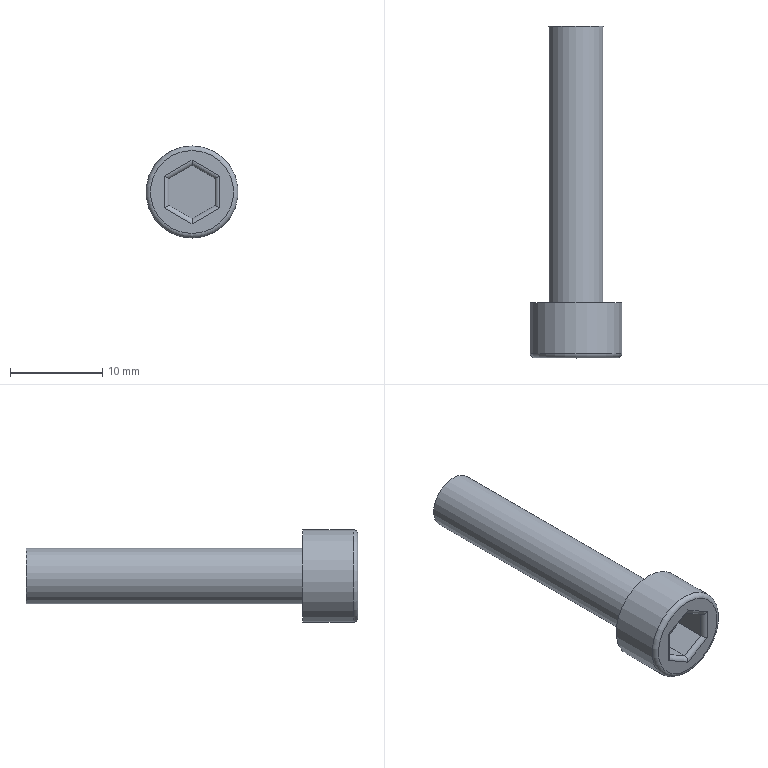Part | STEP file | Tube feed_id34_x_t | 1 solid | 19 faces | box 10 x 36 x 10 mm | volume 1231 mm3 | plane 10 | cylinder 8 | torus 1 | commonest cylinder face diameters 1 x6 6 x1 10 x1